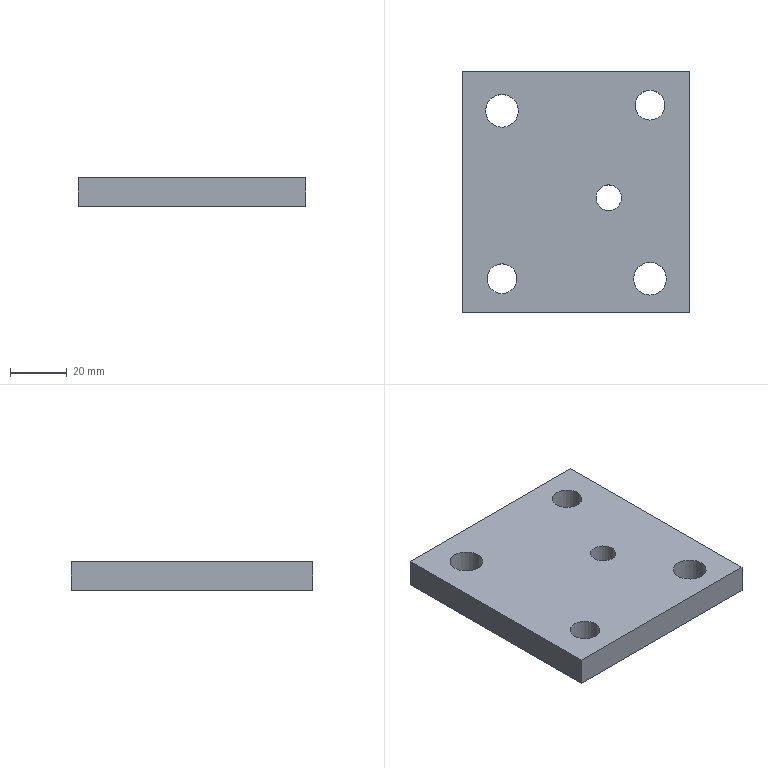Part | NX | features 6 2 | 1 solid | 11 faces | box 80 x 85 x 10 mm | volume 63555 mm3 | plane 6 | cylinder 5 | commonest cylinder face diameters 10.5 x2 11.5 x2 9 x1
STEP:
#1=CARTESIAN_POINT('',(3236.438,86.438,101.));
#2=VERTEX_POINT('',#1);
#3=CARTESIAN_POINT('',(3236.438,1.438,101.));
#4=VERTEX_POINT('',#3);
#5=CARTESIAN_POINT('',(3236.438,41.938,101.));
#6=DIRECTION('',(0.,-1.,0.));
#7=VECTOR('',#6,1000.);
#8=LINE('',#5,#7);
#9=EDGE_CURVE('',#2,#4,#8,.T.);
#10=ORIENTED_EDGE('',*,*,#9,.T.);
#11=CARTESIAN_POINT('',(3236.438,1.438,91.));
#12=VERTEX_POINT('',#11);
#13=CARTESIAN_POINT('',(3236.438,1.438,91.));
#14=DIRECTION('',(0.,0.,1.));
#15=VECTOR('',#14,1000.);
#16=LINE('',#13,#15);
#17=EDGE_CURVE('',#12,#4,#16,.T.);
#18=ORIENTED_EDGE('',*,*,#17,.F.);
#19=CARTESIAN_POINT('',(3236.438,86.438,91.));
#20=VERTEX_POINT('',#19);
#21=CARTESIAN_POINT('',(3236.438,41.938,91.));
#22=DIRECTION('',(0.,-1.,0.));
#23=VECTOR('',#22,1000.);
#24=LINE('',#21,#23);
#25=EDGE_CURVE('',#20,#12,#24,.T.);
#26=ORIENTED_EDGE('',*,*,#25,.F.);
#27=CARTESIAN_POINT('',(3236.438,86.438,91.));
#28=DIRECTION('',(0.,0.,-1.));
#29=VECTOR('',#28,1000.);
#30=LINE('',#27,#29);
#31=EDGE_CURVE('',#2,#20,#30,.T.);
#32=ORIENTED_EDGE('',*,*,#31,.F.);
#33=EDGE_LOOP('',(#10,#18,#26,#32));
#34=FACE_BOUND('',#33,.T.);
#35=CARTESIAN_POINT('',(3236.438,41.938,91.));
#36=DIRECTION('',(-1.,0.,0.));
#37=DIRECTION('',(0.,-1.,0.));
#38=AXIS2_PLACEMENT_3D('',#35,#36,#37);
#39=PLANE('',#38);
#40=ADVANCED_FACE('',(#34),#39,.F.);
#41=CARTESIAN_POINT('',(3156.438,86.438,101.));
#42=VERTEX_POINT('',#41);
#43=CARTESIAN_POINT('',(3186.438,86.438,101.));
#44=DIRECTION('',(1.,0.,0.));
#45=VECTOR('',#44,1000.);
#46=LINE('',#43,#45);
#47=EDGE_CURVE('',#42,#2,#46,.T.);
#48=ORIENTED_EDGE('',*,*,#47,.T.);
#49=ORIENTED_EDGE('',*,*,#31,.T.);
#50=CARTESIAN_POINT('',(3156.438,86.438,91.));
#51=VERTEX_POINT('',#50);
#52=CARTESIAN_POINT('',(3186.438,86.438,91.));
#53=DIRECTION('',(1.,0.,0.));
#54=VECTOR('',#53,1000.);
#55=LINE('',#52,#54);
#56=EDGE_CURVE('',#51,#20,#55,.T.);
#57=ORIENTED_EDGE('',*,*,#56,.F.);
#58=CARTESIAN_POINT('',(3156.438,86.438,91.));
#59=DIRECTION('',(0.,0.,-1.));
#60=VECTOR('',#59,1000.);
#61=LINE('',#58,#60);
#62=EDGE_CURVE('',#42,#51,#61,.T.);
#63=ORIENTED_EDGE('',*,*,#62,.F.);
#64=EDGE_LOOP('',(#48,#49,#57,#63));
#65=FACE_BOUND('',#64,.T.);
#66=CARTESIAN_POINT('',(3186.438,86.438,91.));
#67=DIRECTION('',(0.,-1.,0.));
#68=DIRECTION('',(1.,0.,0.));
#69=AXIS2_PLACEMENT_3D('',#66,#67,#68);
#70=PLANE('',#69);
#71=ADVANCED_FACE('',(#65),#70,.F.);
#72=CARTESIAN_POINT('',(3156.438,1.438,101.));
#73=VERTEX_POINT('',#72);
#74=CARTESIAN_POINT('',(3156.438,41.938,101.));
#75=DIRECTION('',(0.,1.,0.));
#76=VECTOR('',#75,1000.);
#77=LINE('',#74,#76);
#78=EDGE_CURVE('',#73,#42,#77,.T.);
#79=ORIENTED_EDGE('',*,*,#78,.T.);
#80=ORIENTED_EDGE('',*,*,#62,.T.);
#81=CARTESIAN_POINT('',(3156.438,1.438,91.));
#82=VERTEX_POINT('',#81);
#83=CARTESIAN_POINT('',(3156.438,41.938,91.));
#84=DIRECTION('',(0.,1.,0.));
#85=VECTOR('',#84,1000.);
#86=LINE('',#83,#85);
#87=EDGE_CURVE('',#82,#51,#86,.T.);
#88=ORIENTED_EDGE('',*,*,#87,.F.);
#89=CARTESIAN_POINT('',(3156.438,1.438,91.));
#90=DIRECTION('',(0.,0.,-1.));
#91=VECTOR('',#90,1000.);
#92=LINE('',#89,#91);
#93=EDGE_CURVE('',#73,#82,#92,.T.);
#94=ORIENTED_EDGE('',*,*,#93,.F.);
#95=EDGE_LOOP('',(#79,#80,#88,#94));
#96=FACE_BOUND('',#95,.T.);
#97=CARTESIAN_POINT('',(3156.438,41.938,91.));
#98=DIRECTION('',(1.,0.,0.));
#99=DIRECTION('',(0.,1.,0.));
#100=AXIS2_PLACEMENT_3D('',#97,#98,#99);
#101=PLANE('',#100);
#102=ADVANCED_FACE('',(#96),#101,.F.);
#103=CARTESIAN_POINT('',(3170.438,8.188,91.));
#104=VERTEX_POINT('',#103);
#105=CARTESIAN_POINT('',(3170.438,13.438,91.));
#106=DIRECTION('',(0.,0.,-1.));
#107=DIRECTION('',(0.,-1.,0.));
#108=AXIS2_PLACEMENT_3D('',#105,#106,#107);
#109=CIRCLE('',#108,5.25);
#110=EDGE_CURVE('',#104,#104,#109,.T.);
#111=ORIENTED_EDGE('',*,*,#110,.T.);
#112=EDGE_LOOP('',(#111));
#113=FACE_BOUND('',#112,.T.);
#114=CARTESIAN_POINT('',(3170.438,18.688,101.));
#115=VERTEX_POINT('',#114);
#116=CARTESIAN_POINT('',(3170.438,13.438,101.));
#117=DIRECTION('',(0.,0.,1.));
#118=DIRECTION('',(0.,1.,0.));
#119=AXIS2_PLACEMENT_3D('',#116,#117,#118);
#120=CIRCLE('',#119,5.25);
#121=EDGE_CURVE('',#115,#115,#120,.T.);
#122=ORIENTED_EDGE('',*,*,#121,.T.);
#123=EDGE_LOOP('',(#122));
#124=FACE_BOUND('',#123,.T.);
#125=CARTESIAN_POINT('',(3170.438,13.438,91.));
#126=DIRECTION('',(0.,0.,1.));
#127=DIRECTION('',(0.,-1.,0.));
#128=AXIS2_PLACEMENT_3D('',#125,#126,#127);
#129=CYLINDRICAL_SURFACE('',#128,5.25);
#130=ADVANCED_FACE('',(#113,#124),#129,.F.);
#131=CARTESIAN_POINT('',(3222.438,19.188,91.));
#132=VERTEX_POINT('',#131);
#133=CARTESIAN_POINT('',(3222.438,13.438,91.));
#134=DIRECTION('',(0.,0.,1.));
#135=DIRECTION('',(0.,1.,0.));
#136=AXIS2_PLACEMENT_3D('',#133,#134,#135);
#137=CIRCLE('',#136,5.75);
#138=EDGE_CURVE('',#132,#132,#137,.T.);
#139=ORIENTED_EDGE('',*,*,#138,.F.);
#140=EDGE_LOOP('',(#139));
#141=FACE_BOUND('',#140,.T.);
#142=CARTESIAN_POINT('',(3222.438,19.188,101.));
#143=VERTEX_POINT('',#142);
#144=CARTESIAN_POINT('',(3222.438,13.438,101.));
#145=DIRECTION('',(0.,0.,1.));
#146=DIRECTION('',(0.,1.,0.));
#147=AXIS2_PLACEMENT_3D('',#144,#145,#146);
#148=CIRCLE('',#147,5.75);
#149=EDGE_CURVE('',#143,#143,#148,.T.);
#150=ORIENTED_EDGE('',*,*,#149,.T.);
#151=EDGE_LOOP('',(#150));
#152=FACE_BOUND('',#151,.T.);
#153=CARTESIAN_POINT('',(3222.438,13.438,91.));
#154=DIRECTION('',(0.,0.,1.));
#155=DIRECTION('',(0.,-1.,0.));
#156=AXIS2_PLACEMENT_3D('',#153,#154,#155);
#157=CYLINDRICAL_SURFACE('',#156,5.75);
#158=ADVANCED_FACE('',(#141,#152),#157,.F.);
#159=CARTESIAN_POINT('',(3186.438,1.438,91.));
#160=DIRECTION('',(-1.,0.,0.));
#161=VECTOR('',#160,1000.);
#162=LINE('',#159,#161);
#163=EDGE_CURVE('',#12,#82,#162,.T.);
#164=ORIENTED_EDGE('',*,*,#163,.F.);
#165=ORIENTED_EDGE('',*,*,#17,.T.);
#166=CARTESIAN_POINT('',(3186.438,1.438,101.));
#167=DIRECTION('',(-1.,0.,0.));
#168=VECTOR('',#167,1000.);
#169=LINE('',#166,#168);
#170=EDGE_CURVE('',#4,#73,#169,.T.);
#171=ORIENTED_EDGE('',*,*,#170,.T.);
#172=ORIENTED_EDGE('',*,*,#93,.T.);
#173=EDGE_LOOP('',(#164,#165,#171,#172));
#174=FACE_BOUND('',#173,.T.);
#175=CARTESIAN_POINT('',(3186.438,1.438,91.));
#176=DIRECTION('',(0.,1.,0.));
#177=DIRECTION('',(-1.,0.,0.));
#178=AXIS2_PLACEMENT_3D('',#175,#176,#177);
#179=PLANE('',#178);
#180=ADVANCED_FACE('',(#174),#179,.F.);
#181=CARTESIAN_POINT('',(3170.438,78.188,91.));
#182=VERTEX_POINT('',#181);
#183=CARTESIAN_POINT('',(3170.438,72.438,91.));
#184=DIRECTION('',(0.,0.,1.));
#185=DIRECTION('',(0.,1.,0.));
#186=AXIS2_PLACEMENT_3D('',#183,#184,#185);
#187=CIRCLE('',#186,5.75);
#188=EDGE_CURVE('',#182,#182,#187,.T.);
#189=ORIENTED_EDGE('',*,*,#188,.F.);
#190=EDGE_LOOP('',(#189));
#191=FACE_BOUND('',#190,.T.);
#192=CARTESIAN_POINT('',(3170.438,78.188,101.));
#193=VERTEX_POINT('',#192);
#194=CARTESIAN_POINT('',(3170.438,72.438,101.));
#195=DIRECTION('',(0.,0.,1.));
#196=DIRECTION('',(0.,1.,0.));
#197=AXIS2_PLACEMENT_3D('',#194,#195,#196);
#198=CIRCLE('',#197,5.75);
#199=EDGE_CURVE('',#193,#193,#198,.T.);
#200=ORIENTED_EDGE('',*,*,#199,.T.);
#201=EDGE_LOOP('',(#200));
#202=FACE_BOUND('',#201,.T.);
#203=CARTESIAN_POINT('',(3170.438,72.438,91.));
#204=DIRECTION('',(0.,0.,1.));
#205=DIRECTION('',(0.,-1.,0.));
#206=AXIS2_PLACEMENT_3D('',#203,#204,#205);
#207=CYLINDRICAL_SURFACE('',#206,5.75);
#208=ADVANCED_FACE('',(#191,#202),#207,.F.);
#209=CARTESIAN_POINT('',(3222.438,69.188,91.));
#210=VERTEX_POINT('',#209);
#211=CARTESIAN_POINT('',(3222.438,74.438,91.));
#212=DIRECTION('',(0.,0.,-1.));
#213=DIRECTION('',(0.,-1.,0.));
#214=AXIS2_PLACEMENT_3D('',#211,#212,#213);
#215=CIRCLE('',#214,5.25);
#216=EDGE_CURVE('',#210,#210,#215,.T.);
#217=ORIENTED_EDGE('',*,*,#216,.T.);
#218=EDGE_LOOP('',(#217));
#219=FACE_BOUND('',#218,.T.);
#220=CARTESIAN_POINT('',(3222.438,79.688,101.));
#221=VERTEX_POINT('',#220);
#222=CARTESIAN_POINT('',(3222.438,74.438,101.));
#223=DIRECTION('',(0.,0.,1.));
#224=DIRECTION('',(0.,1.,0.));
#225=AXIS2_PLACEMENT_3D('',#222,#223,#224);
#226=CIRCLE('',#225,5.25);
#227=EDGE_CURVE('',#221,#221,#226,.T.);
#228=ORIENTED_EDGE('',*,*,#227,.T.);
#229=EDGE_LOOP('',(#228));
#230=FACE_BOUND('',#229,.T.);
#231=CARTESIAN_POINT('',(3222.438,74.438,91.));
#232=DIRECTION('',(0.,0.,1.));
#233=DIRECTION('',(0.,-1.,0.));
#234=AXIS2_PLACEMENT_3D('',#231,#232,#233);
#235=CYLINDRICAL_SURFACE('',#234,5.25);
#236=ADVANCED_FACE('',(#219,#230),#235,.F.);
#237=CARTESIAN_POINT('',(3207.938,46.438,91.));
#238=VERTEX_POINT('',#237);
#239=CARTESIAN_POINT('',(3207.938,41.938,91.));
#240=DIRECTION('',(0.,0.,-1.));
#241=DIRECTION('',(0.,1.,0.));
#242=AXIS2_PLACEMENT_3D('',#239,#240,#241);
#243=CIRCLE('',#242,4.5);
#244=EDGE_CURVE('',#238,#238,#243,.T.);
#245=ORIENTED_EDGE('',*,*,#244,.T.);
#246=EDGE_LOOP('',(#245));
#247=FACE_BOUND('',#246,.T.);
#248=CARTESIAN_POINT('',(3207.938,46.438,101.));
#249=VERTEX_POINT('',#248);
#250=CARTESIAN_POINT('',(3207.938,41.938,101.));
#251=DIRECTION('',(0.,0.,1.));
#252=DIRECTION('',(0.,1.,0.));
#253=AXIS2_PLACEMENT_3D('',#250,#251,#252);
#254=CIRCLE('',#253,4.5);
#255=EDGE_CURVE('',#249,#249,#254,.T.);
#256=ORIENTED_EDGE('',*,*,#255,.T.);
#257=EDGE_LOOP('',(#256));
#258=FACE_BOUND('',#257,.T.);
#259=CARTESIAN_POINT('',(3207.938,41.938,-119.));
#260=DIRECTION('',(0.,0.,1.));
#261=DIRECTION('',(0.,-1.,0.));
#262=AXIS2_PLACEMENT_3D('',#259,#260,#261);
#263=CYLINDRICAL_SURFACE('',#262,4.5);
#264=ADVANCED_FACE('',(#247,#258),#263,.F.);
#265=ORIENTED_EDGE('',*,*,#216,.F.);
#266=EDGE_LOOP('',(#265));
#267=FACE_BOUND('',#266,.T.);
#268=ORIENTED_EDGE('',*,*,#188,.T.);
#269=EDGE_LOOP('',(#268));
#270=FACE_BOUND('',#269,.T.);
#271=ORIENTED_EDGE('',*,*,#87,.T.);
#272=ORIENTED_EDGE('',*,*,#56,.T.);
#273=ORIENTED_EDGE('',*,*,#25,.T.);
#274=ORIENTED_EDGE('',*,*,#163,.T.);
#275=EDGE_LOOP('',(#271,#272,#273,#274));
#276=FACE_BOUND('',#275,.T.);
#277=ORIENTED_EDGE('',*,*,#138,.T.);
#278=EDGE_LOOP('',(#277));
#279=FACE_BOUND('',#278,.T.);
#280=ORIENTED_EDGE('',*,*,#110,.F.);
#281=EDGE_LOOP('',(#280));
#282=FACE_BOUND('',#281,.T.);
#283=ORIENTED_EDGE('',*,*,#244,.F.);
#284=EDGE_LOOP('',(#283));
#285=FACE_BOUND('',#284,.T.);
#286=CARTESIAN_POINT('',(3186.438,41.938,91.));
#287=DIRECTION('',(0.,0.,1.));
#288=DIRECTION('',(0.,-1.,0.));
#289=AXIS2_PLACEMENT_3D('',#286,#287,#288);
#290=PLANE('',#289);
#291=ADVANCED_FACE('',(#267,#270,#276,#279,#282,#285),#290,.F.);
#292=ORIENTED_EDGE('',*,*,#121,.F.);
#293=EDGE_LOOP('',(#292));
#294=FACE_BOUND('',#293,.T.);
#295=ORIENTED_EDGE('',*,*,#149,.F.);
#296=EDGE_LOOP('',(#295));
#297=FACE_BOUND('',#296,.T.);
#298=ORIENTED_EDGE('',*,*,#170,.F.);
#299=ORIENTED_EDGE('',*,*,#9,.F.);
#300=ORIENTED_EDGE('',*,*,#47,.F.);
#301=ORIENTED_EDGE('',*,*,#78,.F.);
#302=EDGE_LOOP('',(#298,#299,#300,#301));
#303=FACE_BOUND('',#302,.T.);
#304=ORIENTED_EDGE('',*,*,#199,.F.);
#305=EDGE_LOOP('',(#304));
#306=FACE_BOUND('',#305,.T.);
#307=ORIENTED_EDGE('',*,*,#227,.F.);
#308=EDGE_LOOP('',(#307));
#309=FACE_BOUND('',#308,.T.);
#310=ORIENTED_EDGE('',*,*,#255,.F.);
#311=EDGE_LOOP('',(#310));
#312=FACE_BOUND('',#311,.T.);
#313=CARTESIAN_POINT('',(3368.438,1171.938,101.));
#314=DIRECTION('',(0.,0.,1.));
#315=DIRECTION('',(0.,1.,0.));
#316=AXIS2_PLACEMENT_3D('',#313,#314,#315);
#317=PLANE('',#316);
#318=ADVANCED_FACE('',(#294,#297,#303,#306,#309,#312),#317,.T.);
#319=CLOSED_SHELL('',(#40,#71,#102,#130,#158,#180,#208,#236,#264,#291,#318));
#320=MANIFOLD_SOLID_BREP('',#319);
#321=(LENGTH_UNIT()NAMED_UNIT(*)SI_UNIT(.MILLI.,.METRE.));
#322=UNCERTAINTY_MEASURE_WITH_UNIT(LENGTH_MEASURE(0.00001),#321,'','');
#323=(NAMED_UNIT(*)PLANE_ANGLE_UNIT()SI_UNIT($,.RADIAN.));
#324=(NAMED_UNIT(*)SI_UNIT($,.STERADIAN.)SOLID_ANGLE_UNIT());
#325=(GEOMETRIC_REPRESENTATION_CONTEXT(3)GLOBAL_UNCERTAINTY_ASSIGNED_CONTEXT((#322))GLOBAL_UNIT_ASSIGNED_CONTEXT((#321,#323,#324))REPRESENTATION_CONTEXT('',''));
#326=ADVANCED_BREP_SHAPE_REPRESENTATION('',(#320),#325);